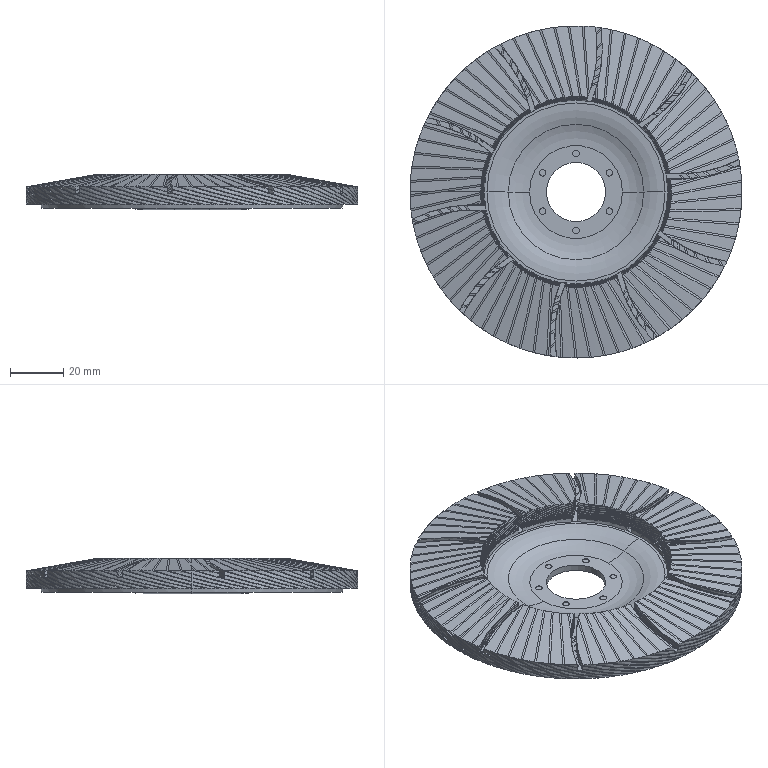Part | SolidWorks | features BaseBody 1, CutThin 1 | 27 solids | 962 faces | box 125 x 125 x 13.257 mm | volume 65573 mm3 | plane 368 | cylinder 316 | cone 270 | torus 8 | commonest cylinder face diameters 103.42 x98 99.42 x97 125 x95 2.5 x24 22.3 x2